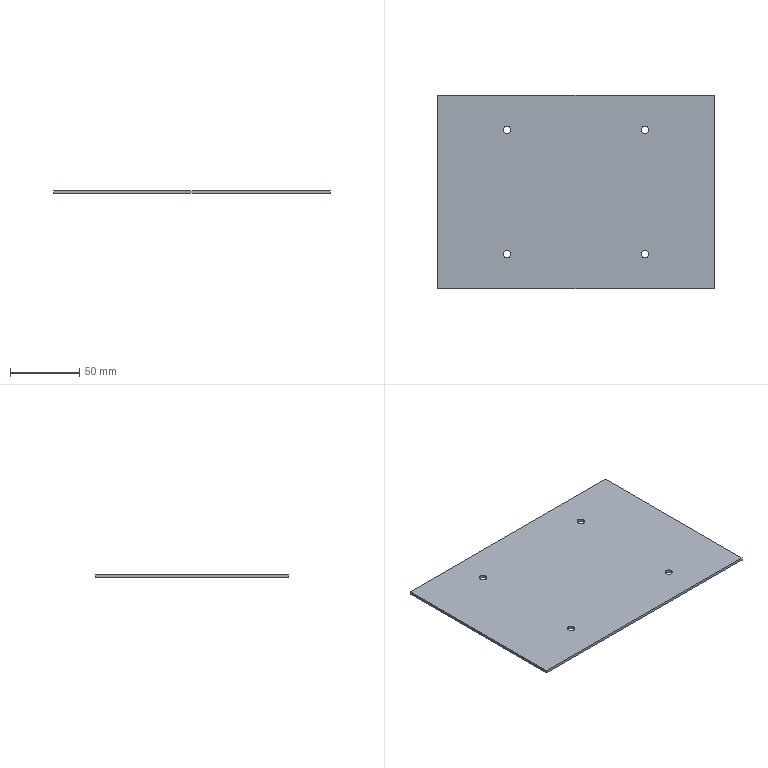Part | STEP file | SX-S36 | 1 solid | 14 faces | box 200 x 140 x 2 mm | volume 55817 mm3 | cylinder 8 | plane 6 | commonest cylinder face diameters 5.4 x8
STEP:
#1=CARTESIAN_POINT('',(0.,0.,0.));
#2=DIRECTION('',(0.,0.,1.));
#3=DIRECTION('',(1.,0.,0.));
#4=AXIS2_PLACEMENT_3D('',#1,#2,#3);
#5=CARTESIAN_POINT('',(-1471.912,1227.706,-2.));
#6=VERTEX_POINT('',#5);
#7=CARTESIAN_POINT('',(-1471.912,1227.706,0.));
#8=VERTEX_POINT('',#7);
#9=CARTESIAN_POINT('',(-1471.912,1227.706,-2.));
#10=DIRECTION('',(0.,0.,1.));
#11=VECTOR('',#10,1.);
#12=LINE('',#9,#11);
#13=CARTESIAN_POINT('',(-1474.612,1227.706,-2.));
#14=DIRECTION('',(0.,0.,1.));
#15=DIRECTION('',(1.,0.,0.));
#16=AXIS2_PLACEMENT_3D('',#13,#14,#15);
#17=CYLINDRICAL_SURFACE('',#16,2.7);
#18=CARTESIAN_POINT('',(6.283,0.));
#19=DIRECTION('',(0.,1.));
#20=VECTOR('',#19,1.);
#21=LINE('',#18,#20);
#22=(GEOMETRIC_REPRESENTATION_CONTEXT(2)PARAMETRIC_REPRESENTATION_CONTEXT()REPRESENTATION_CONTEXT('',''));
#23=DEFINITIONAL_REPRESENTATION('',(#21),#22);
#24=PCURVE('',#17,#23);
#25=CARTESIAN_POINT('',(-1474.612,1227.706,-2.));
#26=DIRECTION('',(0.,0.,1.));
#27=DIRECTION('',(1.,0.,0.));
#28=AXIS2_PLACEMENT_3D('',#25,#26,#27);
#29=CYLINDRICAL_SURFACE('',#28,2.7);
#30=CARTESIAN_POINT('',(0.,0.));
#31=DIRECTION('',(0.,1.));
#32=VECTOR('',#31,1.);
#33=LINE('',#30,#32);
#34=(GEOMETRIC_REPRESENTATION_CONTEXT(2)PARAMETRIC_REPRESENTATION_CONTEXT()REPRESENTATION_CONTEXT('',''));
#35=DEFINITIONAL_REPRESENTATION('',(#33),#34);
#36=PCURVE('',#29,#35);
#37=SURFACE_CURVE('',#12,(#24,#36),.PCURVE_S1.);
#38=EDGE_CURVE('',#6,#8,#37,.T.);
#39=ORIENTED_EDGE('',*,*,#38,.T.);
#40=CARTESIAN_POINT('',(-1477.312,1227.706,0.));
#41=VERTEX_POINT('',#40);
#42=CARTESIAN_POINT('',(-1474.612,1227.706,0.));
#43=DIRECTION('',(0.,0.,1.));
#44=DIRECTION('',(-1.,0.,0.));
#45=AXIS2_PLACEMENT_3D('',#42,#43,#44);
#46=CIRCLE('',#45,2.7);
#47=CARTESIAN_POINT('',(3.142,2.));
#48=DIRECTION('',(1.,0.));
#49=VECTOR('',#48,1.);
#50=LINE('',#47,#49);
#51=(GEOMETRIC_REPRESENTATION_CONTEXT(2)PARAMETRIC_REPRESENTATION_CONTEXT()REPRESENTATION_CONTEXT('',''));
#52=DEFINITIONAL_REPRESENTATION('',(#50),#51);
#53=PCURVE('',#17,#52);
#54=CARTESIAN_POINT('',(0.,0.,0.));
#55=DIRECTION('',(0.,0.,1.));
#56=DIRECTION('',(1.,0.,0.));
#57=AXIS2_PLACEMENT_3D('',#54,#55,#56);
#58=PLANE('',#57);
#59=CARTESIAN_POINT('',(-1474.612,1227.706));
#60=DIRECTION('',(-1.,0.));
#61=AXIS2_PLACEMENT_2D('',#59,#60);
#62=CIRCLE('',#61,2.7);
#63=(GEOMETRIC_REPRESENTATION_CONTEXT(2)PARAMETRIC_REPRESENTATION_CONTEXT()REPRESENTATION_CONTEXT('',''));
#64=DEFINITIONAL_REPRESENTATION('',(#62),#63);
#65=PCURVE('',#58,#64);
#66=SURFACE_CURVE('',#46,(#53,#65),.PCURVE_S1.);
#67=EDGE_CURVE('',#41,#8,#66,.T.);
#68=ORIENTED_EDGE('',*,*,#67,.F.);
#69=CARTESIAN_POINT('',(-1477.312,1227.706,-2.));
#70=VERTEX_POINT('',#69);
#71=CARTESIAN_POINT('',(-1477.312,1227.706,-2.));
#72=DIRECTION('',(0.,0.,1.));
#73=VECTOR('',#72,1.);
#74=LINE('',#71,#73);
#75=CARTESIAN_POINT('',(3.142,0.));
#76=DIRECTION('',(0.,1.));
#77=VECTOR('',#76,1.);
#78=LINE('',#75,#77);
#79=(GEOMETRIC_REPRESENTATION_CONTEXT(2)PARAMETRIC_REPRESENTATION_CONTEXT()REPRESENTATION_CONTEXT('',''));
#80=DEFINITIONAL_REPRESENTATION('',(#78),#79);
#81=PCURVE('',#17,#80);
#82=CARTESIAN_POINT('',(3.142,0.));
#83=DIRECTION('',(0.,1.));
#84=VECTOR('',#83,1.);
#85=LINE('',#82,#84);
#86=(GEOMETRIC_REPRESENTATION_CONTEXT(2)PARAMETRIC_REPRESENTATION_CONTEXT()REPRESENTATION_CONTEXT('',''));
#87=DEFINITIONAL_REPRESENTATION('',(#85),#86);
#88=PCURVE('',#29,#87);
#89=SURFACE_CURVE('',#74,(#81,#88),.PCURVE_S1.);
#90=EDGE_CURVE('',#70,#41,#89,.T.);
#91=ORIENTED_EDGE('',*,*,#90,.F.);
#92=CARTESIAN_POINT('',(-1474.612,1227.706,-2.));
#93=DIRECTION('',(0.,0.,1.));
#94=DIRECTION('',(-1.,0.,0.));
#95=AXIS2_PLACEMENT_3D('',#92,#93,#94);
#96=CIRCLE('',#95,2.7);
#97=CARTESIAN_POINT('',(3.142,0.));
#98=DIRECTION('',(1.,0.));
#99=VECTOR('',#98,1.);
#100=LINE('',#97,#99);
#101=(GEOMETRIC_REPRESENTATION_CONTEXT(2)PARAMETRIC_REPRESENTATION_CONTEXT()REPRESENTATION_CONTEXT('',''));
#102=DEFINITIONAL_REPRESENTATION('',(#100),#101);
#103=PCURVE('',#17,#102);
#104=CARTESIAN_POINT('',(0.,0.,-2.));
#105=DIRECTION('',(0.,0.,1.));
#106=DIRECTION('',(1.,0.,0.));
#107=AXIS2_PLACEMENT_3D('',#104,#105,#106);
#108=PLANE('',#107);
#109=CARTESIAN_POINT('',(-1474.612,1227.706));
#110=DIRECTION('',(-1.,0.));
#111=AXIS2_PLACEMENT_2D('',#109,#110);
#112=CIRCLE('',#111,2.7);
#113=(GEOMETRIC_REPRESENTATION_CONTEXT(2)PARAMETRIC_REPRESENTATION_CONTEXT()REPRESENTATION_CONTEXT('',''));
#114=DEFINITIONAL_REPRESENTATION('',(#112),#113);
#115=PCURVE('',#108,#114);
#116=SURFACE_CURVE('',#96,(#103,#115),.PCURVE_S1.);
#117=EDGE_CURVE('',#70,#6,#116,.T.);
#118=ORIENTED_EDGE('',*,*,#117,.T.);
#119=EDGE_LOOP('',(#39,#68,#91,#118));
#120=FACE_BOUND('',#119,.F.);
#121=ADVANCED_FACE('',(#120),#17,.F.);
#122=CARTESIAN_POINT('',(-1471.912,1137.706,-2.));
#123=VERTEX_POINT('',#122);
#124=CARTESIAN_POINT('',(-1471.912,1137.706,0.));
#125=VERTEX_POINT('',#124);
#126=CARTESIAN_POINT('',(-1471.912,1137.706,-2.));
#127=DIRECTION('',(0.,0.,1.));
#128=VECTOR('',#127,1.);
#129=LINE('',#126,#128);
#130=CARTESIAN_POINT('',(-1474.612,1137.706,-2.));
#131=DIRECTION('',(0.,0.,1.));
#132=DIRECTION('',(1.,0.,0.));
#133=AXIS2_PLACEMENT_3D('',#130,#131,#132);
#134=CYLINDRICAL_SURFACE('',#133,2.7);
#135=CARTESIAN_POINT('',(6.283,0.));
#136=DIRECTION('',(0.,1.));
#137=VECTOR('',#136,1.);
#138=LINE('',#135,#137);
#139=(GEOMETRIC_REPRESENTATION_CONTEXT(2)PARAMETRIC_REPRESENTATION_CONTEXT()REPRESENTATION_CONTEXT('',''));
#140=DEFINITIONAL_REPRESENTATION('',(#138),#139);
#141=PCURVE('',#134,#140);
#142=CARTESIAN_POINT('',(-1474.612,1137.706,-2.));
#143=DIRECTION('',(0.,0.,1.));
#144=DIRECTION('',(1.,0.,0.));
#145=AXIS2_PLACEMENT_3D('',#142,#143,#144);
#146=CYLINDRICAL_SURFACE('',#145,2.7);
#147=CARTESIAN_POINT('',(0.,0.));
#148=DIRECTION('',(0.,1.));
#149=VECTOR('',#148,1.);
#150=LINE('',#147,#149);
#151=(GEOMETRIC_REPRESENTATION_CONTEXT(2)PARAMETRIC_REPRESENTATION_CONTEXT()REPRESENTATION_CONTEXT('',''));
#152=DEFINITIONAL_REPRESENTATION('',(#150),#151);
#153=PCURVE('',#146,#152);
#154=SURFACE_CURVE('',#129,(#141,#153),.PCURVE_S1.);
#155=EDGE_CURVE('',#123,#125,#154,.T.);
#156=ORIENTED_EDGE('',*,*,#155,.T.);
#157=CARTESIAN_POINT('',(-1477.312,1137.706,0.));
#158=VERTEX_POINT('',#157);
#159=CARTESIAN_POINT('',(-1474.612,1137.706,0.));
#160=DIRECTION('',(0.,0.,1.));
#161=DIRECTION('',(1.,0.,0.));
#162=AXIS2_PLACEMENT_3D('',#159,#160,#161);
#163=CIRCLE('',#162,2.7);
#164=CARTESIAN_POINT('',(0.,2.));
#165=DIRECTION('',(1.,0.));
#166=VECTOR('',#165,1.);
#167=LINE('',#164,#166);
#168=(GEOMETRIC_REPRESENTATION_CONTEXT(2)PARAMETRIC_REPRESENTATION_CONTEXT()REPRESENTATION_CONTEXT('',''));
#169=DEFINITIONAL_REPRESENTATION('',(#167),#168);
#170=PCURVE('',#134,#169);
#171=CARTESIAN_POINT('',(-1474.612,1137.706));
#172=DIRECTION('',(1.,0.));
#173=AXIS2_PLACEMENT_2D('',#171,#172);
#174=CIRCLE('',#173,2.7);
#175=(GEOMETRIC_REPRESENTATION_CONTEXT(2)PARAMETRIC_REPRESENTATION_CONTEXT()REPRESENTATION_CONTEXT('',''));
#176=DEFINITIONAL_REPRESENTATION('',(#174),#175);
#177=PCURVE('',#58,#176);
#178=SURFACE_CURVE('',#163,(#170,#177),.PCURVE_S1.);
#179=EDGE_CURVE('',#158,#125,#178,.T.);
#180=ORIENTED_EDGE('',*,*,#179,.F.);
#181=CARTESIAN_POINT('',(-1477.312,1137.706,-2.));
#182=VERTEX_POINT('',#181);
#183=CARTESIAN_POINT('',(-1477.312,1137.706,-2.));
#184=DIRECTION('',(0.,0.,1.));
#185=VECTOR('',#184,1.);
#186=LINE('',#183,#185);
#187=CARTESIAN_POINT('',(3.142,0.));
#188=DIRECTION('',(0.,1.));
#189=VECTOR('',#188,1.);
#190=LINE('',#187,#189);
#191=(GEOMETRIC_REPRESENTATION_CONTEXT(2)PARAMETRIC_REPRESENTATION_CONTEXT()REPRESENTATION_CONTEXT('',''));
#192=DEFINITIONAL_REPRESENTATION('',(#190),#191);
#193=PCURVE('',#134,#192);
#194=CARTESIAN_POINT('',(3.142,0.));
#195=DIRECTION('',(0.,1.));
#196=VECTOR('',#195,1.);
#197=LINE('',#194,#196);
#198=(GEOMETRIC_REPRESENTATION_CONTEXT(2)PARAMETRIC_REPRESENTATION_CONTEXT()REPRESENTATION_CONTEXT('',''));
#199=DEFINITIONAL_REPRESENTATION('',(#197),#198);
#200=PCURVE('',#146,#199);
#201=SURFACE_CURVE('',#186,(#193,#200),.PCURVE_S1.);
#202=EDGE_CURVE('',#182,#158,#201,.T.);
#203=ORIENTED_EDGE('',*,*,#202,.F.);
#204=CARTESIAN_POINT('',(-1474.612,1137.706,-2.));
#205=DIRECTION('',(0.,0.,1.));
#206=DIRECTION('',(1.,0.,0.));
#207=AXIS2_PLACEMENT_3D('',#204,#205,#206);
#208=CIRCLE('',#207,2.7);
#209=CARTESIAN_POINT('',(0.,0.));
#210=DIRECTION('',(1.,0.));
#211=VECTOR('',#210,1.);
#212=LINE('',#209,#211);
#213=(GEOMETRIC_REPRESENTATION_CONTEXT(2)PARAMETRIC_REPRESENTATION_CONTEXT()REPRESENTATION_CONTEXT('',''));
#214=DEFINITIONAL_REPRESENTATION('',(#212),#213);
#215=PCURVE('',#134,#214);
#216=CARTESIAN_POINT('',(-1474.612,1137.706));
#217=DIRECTION('',(1.,0.));
#218=AXIS2_PLACEMENT_2D('',#216,#217);
#219=CIRCLE('',#218,2.7);
#220=(GEOMETRIC_REPRESENTATION_CONTEXT(2)PARAMETRIC_REPRESENTATION_CONTEXT()REPRESENTATION_CONTEXT('',''));
#221=DEFINITIONAL_REPRESENTATION('',(#219),#220);
#222=PCURVE('',#108,#221);
#223=SURFACE_CURVE('',#208,(#215,#222),.PCURVE_S1.);
#224=EDGE_CURVE('',#182,#123,#223,.T.);
#225=ORIENTED_EDGE('',*,*,#224,.T.);
#226=EDGE_LOOP('',(#156,#180,#203,#225));
#227=FACE_BOUND('',#226,.F.);
#228=ADVANCED_FACE('',(#227),#134,.F.);
#229=CARTESIAN_POINT('',(-1571.912,1137.706,-2.));
#230=VERTEX_POINT('',#229);
#231=CARTESIAN_POINT('',(-1571.912,1137.706,0.));
#232=VERTEX_POINT('',#231);
#233=CARTESIAN_POINT('',(-1571.912,1137.706,-2.));
#234=DIRECTION('',(0.,0.,1.));
#235=VECTOR('',#234,1.);
#236=LINE('',#233,#235);
#237=CARTESIAN_POINT('',(-1574.612,1137.706,-2.));
#238=DIRECTION('',(0.,0.,1.));
#239=DIRECTION('',(1.,0.,0.));
#240=AXIS2_PLACEMENT_3D('',#237,#238,#239);
#241=CYLINDRICAL_SURFACE('',#240,2.7);
#242=CARTESIAN_POINT('',(6.283,0.));
#243=DIRECTION('',(0.,1.));
#244=VECTOR('',#243,1.);
#245=LINE('',#242,#244);
#246=(GEOMETRIC_REPRESENTATION_CONTEXT(2)PARAMETRIC_REPRESENTATION_CONTEXT()REPRESENTATION_CONTEXT('',''));
#247=DEFINITIONAL_REPRESENTATION('',(#245),#246);
#248=PCURVE('',#241,#247);
#249=CARTESIAN_POINT('',(-1574.612,1137.706,-2.));
#250=DIRECTION('',(0.,0.,1.));
#251=DIRECTION('',(1.,0.,0.));
#252=AXIS2_PLACEMENT_3D('',#249,#250,#251);
#253=CYLINDRICAL_SURFACE('',#252,2.7);
#254=CARTESIAN_POINT('',(0.,0.));
#255=DIRECTION('',(0.,1.));
#256=VECTOR('',#255,1.);
#257=LINE('',#254,#256);
#258=(GEOMETRIC_REPRESENTATION_CONTEXT(2)PARAMETRIC_REPRESENTATION_CONTEXT()REPRESENTATION_CONTEXT('',''));
#259=DEFINITIONAL_REPRESENTATION('',(#257),#258);
#260=PCURVE('',#253,#259);
#261=SURFACE_CURVE('',#236,(#248,#260),.PCURVE_S1.);
#262=EDGE_CURVE('',#230,#232,#261,.T.);
#263=ORIENTED_EDGE('',*,*,#262,.T.);
#264=CARTESIAN_POINT('',(-1577.312,1137.706,0.));
#265=VERTEX_POINT('',#264);
#266=CARTESIAN_POINT('',(-1574.612,1137.706,0.));
#267=DIRECTION('',(0.,0.,1.));
#268=DIRECTION('',(-1.,0.,0.));
#269=AXIS2_PLACEMENT_3D('',#266,#267,#268);
#270=CIRCLE('',#269,2.7);
#271=CARTESIAN_POINT('',(3.142,2.));
#272=DIRECTION('',(1.,0.));
#273=VECTOR('',#272,1.);
#274=LINE('',#271,#273);
#275=(GEOMETRIC_REPRESENTATION_CONTEXT(2)PARAMETRIC_REPRESENTATION_CONTEXT()REPRESENTATION_CONTEXT('',''));
#276=DEFINITIONAL_REPRESENTATION('',(#274),#275);
#277=PCURVE('',#241,#276);
#278=CARTESIAN_POINT('',(-1574.612,1137.706));
#279=DIRECTION('',(-1.,0.));
#280=AXIS2_PLACEMENT_2D('',#278,#279);
#281=CIRCLE('',#280,2.7);
#282=(GEOMETRIC_REPRESENTATION_CONTEXT(2)PARAMETRIC_REPRESENTATION_CONTEXT()REPRESENTATION_CONTEXT('',''));
#283=DEFINITIONAL_REPRESENTATION('',(#281),#282);
#284=PCURVE('',#58,#283);
#285=SURFACE_CURVE('',#270,(#277,#284),.PCURVE_S1.);
#286=EDGE_CURVE('',#265,#232,#285,.T.);
#287=ORIENTED_EDGE('',*,*,#286,.F.);
#288=CARTESIAN_POINT('',(-1577.312,1137.706,-2.));
#289=VERTEX_POINT('',#288);
#290=CARTESIAN_POINT('',(-1577.312,1137.706,-2.));
#291=DIRECTION('',(0.,0.,1.));
#292=VECTOR('',#291,1.);
#293=LINE('',#290,#292);
#294=CARTESIAN_POINT('',(3.142,0.));
#295=DIRECTION('',(0.,1.));
#296=VECTOR('',#295,1.);
#297=LINE('',#294,#296);
#298=(GEOMETRIC_REPRESENTATION_CONTEXT(2)PARAMETRIC_REPRESENTATION_CONTEXT()REPRESENTATION_CONTEXT('',''));
#299=DEFINITIONAL_REPRESENTATION('',(#297),#298);
#300=PCURVE('',#241,#299);
#301=CARTESIAN_POINT('',(3.142,0.));
#302=DIRECTION('',(0.,1.));
#303=VECTOR('',#302,1.);
#304=LINE('',#301,#303);
#305=(GEOMETRIC_REPRESENTATION_CONTEXT(2)PARAMETRIC_REPRESENTATION_CONTEXT()REPRESENTATION_CONTEXT('',''));
#306=DEFINITIONAL_REPRESENTATION('',(#304),#305);
#307=PCURVE('',#253,#306);
#308=SURFACE_CURVE('',#293,(#300,#307),.PCURVE_S1.);
#309=EDGE_CURVE('',#289,#265,#308,.T.);
#310=ORIENTED_EDGE('',*,*,#309,.F.);
#311=CARTESIAN_POINT('',(-1574.612,1137.706,-2.));
#312=DIRECTION('',(0.,0.,1.));
#313=DIRECTION('',(-1.,0.,0.));
#314=AXIS2_PLACEMENT_3D('',#311,#312,#313);
#315=CIRCLE('',#314,2.7);
#316=CARTESIAN_POINT('',(3.142,0.));
#317=DIRECTION('',(1.,0.));
#318=VECTOR('',#317,1.);
#319=LINE('',#316,#318);
#320=(GEOMETRIC_REPRESENTATION_CONTEXT(2)PARAMETRIC_REPRESENTATION_CONTEXT()REPRESENTATION_CONTEXT('',''));
#321=DEFINITIONAL_REPRESENTATION('',(#319),#320);
#322=PCURVE('',#241,#321);
#323=CARTESIAN_POINT('',(-1574.612,1137.706));
#324=DIRECTION('',(-1.,0.));
#325=AXIS2_PLACEMENT_2D('',#323,#324);
#326=CIRCLE('',#325,2.7);
#327=(GEOMETRIC_REPRESENTATION_CONTEXT(2)PARAMETRIC_REPRESENTATION_CONTEXT()REPRESENTATION_CONTEXT('',''));
#328=DEFINITIONAL_REPRESENTATION('',(#326),#327);
#329=PCURVE('',#108,#328);
#330=SURFACE_CURVE('',#315,(#322,#329),.PCURVE_S1.);
#331=EDGE_CURVE('',#289,#230,#330,.T.);
#332=ORIENTED_EDGE('',*,*,#331,.T.);
#333=EDGE_LOOP('',(#263,#287,#310,#332));
#334=FACE_BOUND('',#333,.F.);
#335=ADVANCED_FACE('',(#334),#241,.F.);
#336=CARTESIAN_POINT('',(-1571.912,1227.706,-2.));
#337=VERTEX_POINT('',#336);
#338=CARTESIAN_POINT('',(-1571.912,1227.706,0.));
#339=VERTEX_POINT('',#338);
#340=CARTESIAN_POINT('',(-1571.912,1227.706,-2.));
#341=DIRECTION('',(0.,0.,1.));
#342=VECTOR('',#341,1.);
#343=LINE('',#340,#342);
#344=CARTESIAN_POINT('',(-1574.612,1227.706,-2.));
#345=DIRECTION('',(0.,0.,1.));
#346=DIRECTION('',(1.,0.,0.));
#347=AXIS2_PLACEMENT_3D('',#344,#345,#346);
#348=CYLINDRICAL_SURFACE('',#347,2.7);
#349=CARTESIAN_POINT('',(6.283,0.));
#350=DIRECTION('',(0.,1.));
#351=VECTOR('',#350,1.);
#352=LINE('',#349,#351);
#353=(GEOMETRIC_REPRESENTATION_CONTEXT(2)PARAMETRIC_REPRESENTATION_CONTEXT()REPRESENTATION_CONTEXT('',''));
#354=DEFINITIONAL_REPRESENTATION('',(#352),#353);
#355=PCURVE('',#348,#354);
#356=CARTESIAN_POINT('',(-1574.612,1227.706,-2.));
#357=DIRECTION('',(0.,0.,1.));
#358=DIRECTION('',(1.,0.,0.));
#359=AXIS2_PLACEMENT_3D('',#356,#357,#358);
#360=CYLINDRICAL_SURFACE('',#359,2.7);
#361=CARTESIAN_POINT('',(0.,0.));
#362=DIRECTION('',(0.,1.));
#363=VECTOR('',#362,1.);
#364=LINE('',#361,#363);
#365=(GEOMETRIC_REPRESENTATION_CONTEXT(2)PARAMETRIC_REPRESENTATION_CONTEXT()REPRESENTATION_CONTEXT('',''));
#366=DEFINITIONAL_REPRESENTATION('',(#364),#365);
#367=PCURVE('',#360,#366);
#368=SURFACE_CURVE('',#343,(#355,#367),.PCURVE_S1.);
#369=EDGE_CURVE('',#337,#339,#368,.T.);
#370=ORIENTED_EDGE('',*,*,#369,.T.);
#371=CARTESIAN_POINT('',(-1577.312,1227.706,0.));
#372=VERTEX_POINT('',#371);
#373=CARTESIAN_POINT('',(-1574.612,1227.706,0.));
#374=DIRECTION('',(0.,0.,1.));
#375=DIRECTION('',(1.,0.,0.));
#376=AXIS2_PLACEMENT_3D('',#373,#374,#375);
#377=CIRCLE('',#376,2.7);
#378=CARTESIAN_POINT('',(0.,2.));
#379=DIRECTION('',(1.,0.));
#380=VECTOR('',#379,1.);
#381=LINE('',#378,#380);
#382=(GEOMETRIC_REPRESENTATION_CONTEXT(2)PARAMETRIC_REPRESENTATION_CONTEXT()REPRESENTATION_CONTEXT('',''));
#383=DEFINITIONAL_REPRESENTATION('',(#381),#382);
#384=PCURVE('',#348,#383);
#385=CARTESIAN_POINT('',(-1574.612,1227.706));
#386=DIRECTION('',(1.,0.));
#387=AXIS2_PLACEMENT_2D('',#385,#386);
#388=CIRCLE('',#387,2.7);
#389=(GEOMETRIC_REPRESENTATION_CONTEXT(2)PARAMETRIC_REPRESENTATION_CONTEXT()REPRESENTATION_CONTEXT('',''));
#390=DEFINITIONAL_REPRESENTATION('',(#388),#389);
#391=PCURVE('',#58,#390);
#392=SURFACE_CURVE('',#377,(#384,#391),.PCURVE_S1.);
#393=EDGE_CURVE('',#372,#339,#392,.T.);
#394=ORIENTED_EDGE('',*,*,#393,.F.);
#395=CARTESIAN_POINT('',(-1577.312,1227.706,-2.));
#396=VERTEX_POINT('',#395);
#397=CARTESIAN_POINT('',(-1577.312,1227.706,-2.));
#398=DIRECTION('',(0.,0.,1.));
#399=VECTOR('',#398,1.);
#400=LINE('',#397,#399);
#401=CARTESIAN_POINT('',(3.142,0.));
#402=DIRECTION('',(0.,1.));
#403=VECTOR('',#402,1.);
#404=LINE('',#401,#403);
#405=(GEOMETRIC_REPRESENTATION_CONTEXT(2)PARAMETRIC_REPRESENTATION_CONTEXT()REPRESENTATION_CONTEXT('',''));
#406=DEFINITIONAL_REPRESENTATION('',(#404),#405);
#407=PCURVE('',#348,#406);
#408=CARTESIAN_POINT('',(3.142,0.));
#409=DIRECTION('',(0.,1.));
#410=VECTOR('',#409,1.);
#411=LINE('',#408,#410);
#412=(GEOMETRIC_REPRESENTATION_CONTEXT(2)PARAMETRIC_REPRESENTATION_CONTEXT()REPRESENTATION_CONTEXT('',''));
#413=DEFINITIONAL_REPRESENTATION('',(#411),#412);
#414=PCURVE('',#360,#413);
#415=SURFACE_CURVE('',#400,(#407,#414),.PCURVE_S1.);
#416=EDGE_CURVE('',#396,#372,#415,.T.);
#417=ORIENTED_EDGE('',*,*,#416,.F.);
#418=CARTESIAN_POINT('',(-1574.612,1227.706,-2.));
#419=DIRECTION('',(0.,0.,1.));
#420=DIRECTION('',(1.,0.,0.));
#421=AXIS2_PLACEMENT_3D('',#418,#419,#420);
#422=CIRCLE('',#421,2.7);
#423=CARTESIAN_POINT('',(0.,0.));
#424=DIRECTION('',(1.,0.));
#425=VECTOR('',#424,1.);
#426=LINE('',#423,#425);
#427=(GEOMETRIC_REPRESENTATION_CONTEXT(2)PARAMETRIC_REPRESENTATION_CONTEXT()REPRESENTATION_CONTEXT('',''));
#428=DEFINITIONAL_REPRESENTATION('',(#426),#427);
#429=PCURVE('',#348,#428);
#430=CARTESIAN_POINT('',(-1574.612,1227.706));
#431=DIRECTION('',(1.,0.));
#432=AXIS2_PLACEMENT_2D('',#430,#431);
#433=CIRCLE('',#432,2.7);
#434=(GEOMETRIC_REPRESENTATION_CONTEXT(2)PARAMETRIC_REPRESENTATION_CONTEXT()REPRESENTATION_CONTEXT('',''));
#435=DEFINITIONAL_REPRESENTATION('',(#433),#434);
#436=PCURVE('',#108,#435);
#437=SURFACE_CURVE('',#422,(#429,#436),.PCURVE_S1.);
#438=EDGE_CURVE('',#396,#337,#437,.T.);
#439=ORIENTED_EDGE('',*,*,#438,.T.);
#440=EDGE_LOOP('',(#370,#394,#417,#439));
#441=FACE_BOUND('',#440,.F.);
#442=ADVANCED_FACE('',(#441),#348,.F.);
#443=CARTESIAN_POINT('',(-1624.612,1252.706,0.));
#444=VERTEX_POINT('',#443);
#445=CARTESIAN_POINT('',(-1624.612,1112.706,0.));
#446=VERTEX_POINT('',#445);
#447=CARTESIAN_POINT('',(-1624.612,1252.706,0.));
#448=DIRECTION('',(0.,-1.,0.));
#449=VECTOR('',#448,1.);
#450=LINE('',#447,#449);
#451=CARTESIAN_POINT('',(-1624.612,1252.706,-2.));
#452=DIRECTION('',(-1.,0.,0.));
#453=DIRECTION('',(0.,0.,1.));
#454=AXIS2_PLACEMENT_3D('',#451,#452,#453);
#455=PLANE('',#454);
#456=CARTESIAN_POINT('',(2.,0.));
#457=DIRECTION('',(0.,-1.));
#458=VECTOR('',#457,1.);
#459=LINE('',#456,#458);
#460=(GEOMETRIC_REPRESENTATION_CONTEXT(2)PARAMETRIC_REPRESENTATION_CONTEXT()REPRESENTATION_CONTEXT('',''));
#461=DEFINITIONAL_REPRESENTATION('',(#459),#460);
#462=PCURVE('',#455,#461);
#463=CARTESIAN_POINT('',(-1624.612,1252.706));
#464=DIRECTION('',(0.,-1.));
#465=VECTOR('',#464,1.);
#466=LINE('',#463,#465);
#467=(GEOMETRIC_REPRESENTATION_CONTEXT(2)PARAMETRIC_REPRESENTATION_CONTEXT()REPRESENTATION_CONTEXT('',''));
#468=DEFINITIONAL_REPRESENTATION('',(#466),#467);
#469=PCURVE('',#58,#468);
#470=SURFACE_CURVE('',#450,(#462,#469),.PCURVE_S1.);
#471=EDGE_CURVE('',#444,#446,#470,.T.);
#472=ORIENTED_EDGE('',*,*,#471,.F.);
#473=CARTESIAN_POINT('',(-1624.612,1252.706,-2.));
#474=VERTEX_POINT('',#473);
#475=CARTESIAN_POINT('',(-1624.612,1252.706,-2.));
#476=DIRECTION('',(0.,0.,1.));
#477=VECTOR('',#476,1.);
#478=LINE('',#475,#477);
#479=CARTESIAN_POINT('',(0.,0.));
#480=DIRECTION('',(1.,0.));
#481=VECTOR('',#480,1.);
#482=LINE('',#479,#481);
#483=(GEOMETRIC_REPRESENTATION_CONTEXT(2)PARAMETRIC_REPRESENTATION_CONTEXT()REPRESENTATION_CONTEXT('',''));
#484=DEFINITIONAL_REPRESENTATION('',(#482),#483);
#485=PCURVE('',#455,#484);
#486=CARTESIAN_POINT('',(-1624.612,1252.706,-2.));
#487=DIRECTION('',(0.,1.,0.));
#488=DIRECTION('',(0.,0.,1.));
#489=AXIS2_PLACEMENT_3D('',#486,#487,#488);
#490=PLANE('',#489);
#491=CARTESIAN_POINT('',(0.,0.));
#492=DIRECTION('',(1.,0.));
#493=VECTOR('',#492,1.);
#494=LINE('',#491,#493);
#495=(GEOMETRIC_REPRESENTATION_CONTEXT(2)PARAMETRIC_REPRESENTATION_CONTEXT()REPRESENTATION_CONTEXT('',''));
#496=DEFINITIONAL_REPRESENTATION('',(#494),#495);
#497=PCURVE('',#490,#496);
#498=SURFACE_CURVE('',#478,(#485,#497),.PCURVE_S1.);
#499=EDGE_CURVE('',#474,#444,#498,.T.);
#500=ORIENTED_EDGE('',*,*,#499,.F.);
#501=CARTESIAN_POINT('',(-1624.612,1112.706,-2.));
#502=VERTEX_POINT('',#501);
#503=CARTESIAN_POINT('',(-1624.612,1252.706,-2.));
#504=DIRECTION('',(0.,-1.,0.));
#505=VECTOR('',#504,1.);
#506=LINE('',#503,#505);
#507=CARTESIAN_POINT('',(0.,0.));
#508=DIRECTION('',(0.,-1.));
#509=VECTOR('',#508,1.);
#510=LINE('',#507,#509);
#511=(GEOMETRIC_REPRESENTATION_CONTEXT(2)PARAMETRIC_REPRESENTATION_CONTEXT()REPRESENTATION_CONTEXT('',''));
#512=DEFINITIONAL_REPRESENTATION('',(#510),#511);
#513=PCURVE('',#455,#512);
#514=CARTESIAN_POINT('',(-1624.612,1252.706));
#515=DIRECTION('',(0.,-1.));
#516=VECTOR('',#515,1.);
#517=LINE('',#514,#516);
#518=(GEOMETRIC_REPRESENTATION_CONTEXT(2)PARAMETRIC_REPRESENTATION_CONTEXT()REPRESENTATION_CONTEXT('',''));
#519=DEFINITIONAL_REPRESENTATION('',(#517),#518);
#520=PCURVE('',#108,#519);
#521=SURFACE_CURVE('',#506,(#513,#520),.PCURVE_S1.);
#522=EDGE_CURVE('',#474,#502,#521,.T.);
#523=ORIENTED_EDGE('',*,*,#522,.T.);
#524=CARTESIAN_POINT('',(-1624.612,1112.706,-2.));
#525=DIRECTION('',(0.,0.,1.));
#526=VECTOR('',#525,1.);
#527=LINE('',#524,#526);
#528=CARTESIAN_POINT('',(0.,-140.));
#529=DIRECTION('',(1.,0.));
#530=VECTOR('',#529,1.);
#531=LINE('',#528,#530);
#532=(GEOMETRIC_REPRESENTATION_CONTEXT(2)PARAMETRIC_REPRESENTATION_CONTEXT()REPRESENTATION_CONTEXT('',''));
#533=DEFINITIONAL_REPRESENTATION('',(#531),#532);
#534=PCURVE('',#455,#533);
#535=CARTESIAN_POINT('',(-1624.612,1112.706,-2.));
#536=DIRECTION('',(0.,-1.,0.));
#537=DIRECTION('',(0.,0.,-1.));
#538=AXIS2_PLACEMENT_3D('',#535,#536,#537);
#539=PLANE('',#538);
#540=CARTESIAN_POINT('',(0.,0.));
#541=DIRECTION('',(-1.,0.));
#542=VECTOR('',#541,1.);
#543=LINE('',#540,#542);
#544=(GEOMETRIC_REPRESENTATION_CONTEXT(2)PARAMETRIC_REPRESENTATION_CONTEXT()REPRESENTATION_CONTEXT('',''));
#545=DEFINITIONAL_REPRESENTATION('',(#543),#544);
#546=PCURVE('',#539,#545);
#547=SURFACE_CURVE('',#527,(#534,#546),.PCURVE_S1.);
#548=EDGE_CURVE('',#502,#446,#547,.T.);
#549=ORIENTED_EDGE('',*,*,#548,.T.);
#550=EDGE_LOOP('',(#472,#500,#523,#549));
#551=FACE_BOUND('',#550,.T.);
#552=ADVANCED_FACE('',(#551),#455,.T.);
#553=CARTESIAN_POINT('',(-1424.612,1252.706,0.));
#554=VERTEX_POINT('',#553);
#555=CARTESIAN_POINT('',(-1624.612,1252.706,0.));
#556=DIRECTION('',(-1.,0.,0.));
#557=VECTOR('',#556,1.);
#558=LINE('',#555,#557);
#559=CARTESIAN_POINT('',(2.,0.));
#560=DIRECTION('',(0.,-1.));
#561=VECTOR('',#560,1.);
#562=LINE('',#559,#561);
#563=(GEOMETRIC_REPRESENTATION_CONTEXT(2)PARAMETRIC_REPRESENTATION_CONTEXT()REPRESENTATION_CONTEXT('',''));
#564=DEFINITIONAL_REPRESENTATION('',(#562),#563);
#565=PCURVE('',#490,#564);
#566=CARTESIAN_POINT('',(-1624.612,1252.706));
#567=DIRECTION('',(-1.,0.));
#568=VECTOR('',#567,1.);
#569=LINE('',#566,#568);
#570=(GEOMETRIC_REPRESENTATION_CONTEXT(2)PARAMETRIC_REPRESENTATION_CONTEXT()REPRESENTATION_CONTEXT('',''));
#571=DEFINITIONAL_REPRESENTATION('',(#569),#570);
#572=PCURVE('',#58,#571);
#573=SURFACE_CURVE('',#558,(#565,#572),.PCURVE_S1.);
#574=EDGE_CURVE('',#554,#444,#573,.T.);
#575=ORIENTED_EDGE('',*,*,#574,.F.);
#576=CARTESIAN_POINT('',(-1424.612,1252.706,-2.));
#577=VERTEX_POINT('',#576);
#578=CARTESIAN_POINT('',(-1424.612,1252.706,-2.));
#579=DIRECTION('',(0.,0.,1.));
#580=VECTOR('',#579,1.);
#581=LINE('',#578,#580);
#582=CARTESIAN_POINT('',(0.,200.));
#583=DIRECTION('',(1.,0.));
#584=VECTOR('',#583,1.);
#585=LINE('',#582,#584);
#586=(GEOMETRIC_REPRESENTATION_CONTEXT(2)PARAMETRIC_REPRESENTATION_CONTEXT()REPRESENTATION_CONTEXT('',''));
#587=DEFINITIONAL_REPRESENTATION('',(#585),#586);
#588=PCURVE('',#490,#587);
#589=CARTESIAN_POINT('',(-1424.612,1252.706,-2.));
#590=DIRECTION('',(1.,0.,0.));
#591=DIRECTION('',(0.,0.,-1.));
#592=AXIS2_PLACEMENT_3D('',#589,#590,#591);
#593=PLANE('',#592);
#594=CARTESIAN_POINT('',(0.,0.));
#595=DIRECTION('',(-1.,0.));
#596=VECTOR('',#595,1.);
#597=LINE('',#594,#596);
#598=(GEOMETRIC_REPRESENTATION_CONTEXT(2)PARAMETRIC_REPRESENTATION_CONTEXT()REPRESENTATION_CONTEXT('',''));
#599=DEFINITIONAL_REPRESENTATION('',(#597),#598);
#600=PCURVE('',#593,#599);
#601=SURFACE_CURVE('',#581,(#588,#600),.PCURVE_S1.);
#602=EDGE_CURVE('',#577,#554,#601,.T.);
#603=ORIENTED_EDGE('',*,*,#602,.F.);
#604=CARTESIAN_POINT('',(-1624.612,1252.706,-2.));
#605=DIRECTION('',(-1.,0.,0.));
#606=VECTOR('',#605,1.);
#607=LINE('',#604,#606);
#608=CARTESIAN_POINT('',(0.,0.));
#609=DIRECTION('',(0.,-1.));
#610=VECTOR('',#609,1.);
#611=LINE('',#608,#610);
#612=(GEOMETRIC_REPRESENTATION_CONTEXT(2)PARAMETRIC_REPRESENTATION_CONTEXT()REPRESENTATION_CONTEXT('',''));
#613=DEFINITIONAL_REPRESENTATION('',(#611),#612);
#614=PCURVE('',#490,#613);
#615=CARTESIAN_POINT('',(-1624.612,1252.706));
#616=DIRECTION('',(-1.,0.));
#617=VECTOR('',#616,1.);
#618=LINE('',#615,#617);
#619=(GEOMETRIC_REPRESENTATION_CONTEXT(2)PARAMETRIC_REPRESENTATION_CONTEXT()REPRESENTATION_CONTEXT('',''));
#620=DEFINITIONAL_REPRESENTATION('',(#618),#619);
#621=PCURVE('',#108,#620);
#622=SURFACE_CURVE('',#607,(#614,#621),.PCURVE_S1.);
#623=EDGE_CURVE('',#577,#474,#622,.T.);
#624=ORIENTED_EDGE('',*,*,#623,.T.);
#625=ORIENTED_EDGE('',*,*,#499,.T.);
#626=EDGE_LOOP('',(#575,#603,#624,#625));
#627=FACE_BOUND('',#626,.T.);
#628=ADVANCED_FACE('',(#627),#490,.T.);
#629=CARTESIAN_POINT('',(-1424.612,1112.706,0.));
#630=VERTEX_POINT('',#629);
#631=CARTESIAN_POINT('',(-1424.612,1252.706,0.));
#632=DIRECTION('',(0.,1.,0.));
#633=VECTOR('',#632,1.);
#634=LINE('',#631,#633);
#635=CARTESIAN_POINT('',(-2.,0.));
#636=DIRECTION('',(0.,1.));
#637=VECTOR('',#636,1.);
#638=LINE('',#635,#637);
#639=(GEOMETRIC_REPRESENTATION_CONTEXT(2)PARAMETRIC_REPRESENTATION_CONTEXT()REPRESENTATION_CONTEXT('',''));
#640=DEFINITIONAL_REPRESENTATION('',(#638),#639);
#641=PCURVE('',#593,#640);
#642=CARTESIAN_POINT('',(-1424.612,1252.706));
#643=DIRECTION('',(0.,1.));
#644=VECTOR('',#643,1.);
#645=LINE('',#642,#644);
#646=(GEOMETRIC_REPRESENTATION_CONTEXT(2)PARAMETRIC_REPRESENTATION_CONTEXT()REPRESENTATION_CONTEXT('',''));
#647=DEFINITIONAL_REPRESENTATION('',(#645),#646);
#648=PCURVE('',#58,#647);
#649=SURFACE_CURVE('',#634,(#641,#648),.PCURVE_S1.);
#650=EDGE_CURVE('',#630,#554,#649,.T.);
#651=ORIENTED_EDGE('',*,*,#650,.F.);
#652=CARTESIAN_POINT('',(-1424.612,1112.706,-2.));
#653=VERTEX_POINT('',#652);
#654=CARTESIAN_POINT('',(-1424.612,1112.706,-2.));
#655=DIRECTION('',(0.,0.,1.));
#656=VECTOR('',#655,1.);
#657=LINE('',#654,#656);
#658=CARTESIAN_POINT('',(0.,-140.));
#659=DIRECTION('',(-1.,0.));
#660=VECTOR('',#659,1.);
#661=LINE('',#658,#660);
#662=(GEOMETRIC_REPRESENTATION_CONTEXT(2)PARAMETRIC_REPRESENTATION_CONTEXT()REPRESENTATION_CONTEXT('',''));
#663=DEFINITIONAL_REPRESENTATION('',(#661),#662);
#664=PCURVE('',#593,#663);
#665=CARTESIAN_POINT('',(0.,200.));
#666=DIRECTION('',(-1.,0.));
#667=VECTOR('',#666,1.);
#668=LINE('',#665,#667);
#669=(GEOMETRIC_REPRESENTATION_CONTEXT(2)PARAMETRIC_REPRESENTATION_CONTEXT()REPRESENTATION_CONTEXT('',''));
#670=DEFINITIONAL_REPRESENTATION('',(#668),#669);
#671=PCURVE('',#539,#670);
#672=SURFACE_CURVE('',#657,(#664,#671),.PCURVE_S1.);
#673=EDGE_CURVE('',#653,#630,#672,.T.);
#674=ORIENTED_EDGE('',*,*,#673,.F.);
#675=CARTESIAN_POINT('',(-1424.612,1252.706,-2.));
#676=DIRECTION('',(0.,1.,0.));
#677=VECTOR('',#676,1.);
#678=LINE('',#675,#677);
#679=CARTESIAN_POINT('',(0.,0.));
#680=DIRECTION('',(0.,1.));
#681=VECTOR('',#680,1.);
#682=LINE('',#679,#681);
#683=(GEOMETRIC_REPRESENTATION_CONTEXT(2)PARAMETRIC_REPRESENTATION_CONTEXT()REPRESENTATION_CONTEXT('',''));
#684=DEFINITIONAL_REPRESENTATION('',(#682),#683);
#685=PCURVE('',#593,#684);
#686=CARTESIAN_POINT('',(-1424.612,1252.706));
#687=DIRECTION('',(0.,1.));
#688=VECTOR('',#687,1.);
#689=LINE('',#686,#688);
#690=(GEOMETRIC_REPRESENTATION_CONTEXT(2)PARAMETRIC_REPRESENTATION_CONTEXT()REPRESENTATION_CONTEXT('',''));
#691=DEFINITIONAL_REPRESENTATION('',(#689),#690);
#692=PCURVE('',#108,#691);
#693=SURFACE_CURVE('',#678,(#685,#692),.PCURVE_S1.);
#694=EDGE_CURVE('',#653,#577,#693,.T.);
#695=ORIENTED_EDGE('',*,*,#694,.T.);
#696=ORIENTED_EDGE('',*,*,#602,.T.);
#697=EDGE_LOOP('',(#651,#674,#695,#696));
#698=FACE_BOUND('',#697,.T.);
#699=ADVANCED_FACE('',(#698),#593,.T.);
#700=CARTESIAN_POINT('',(-1624.612,1112.706,0.));
#701=DIRECTION('',(1.,0.,0.));
#702=VECTOR('',#701,1.);
#703=LINE('',#700,#702);
#704=CARTESIAN_POINT('',(-2.,0.));
#705=DIRECTION('',(0.,1.));
#706=VECTOR('',#705,1.);
#707=LINE('',#704,#706);
#708=(GEOMETRIC_REPRESENTATION_CONTEXT(2)PARAMETRIC_REPRESENTATION_CONTEXT()REPRESENTATION_CONTEXT('',''));
#709=DEFINITIONAL_REPRESENTATION('',(#707),#708);
#710=PCURVE('',#539,#709);
#711=CARTESIAN_POINT('',(-1624.612,1112.706));
#712=DIRECTION('',(1.,0.));
#713=VECTOR('',#712,1.);
#714=LINE('',#711,#713);
#715=(GEOMETRIC_REPRESENTATION_CONTEXT(2)PARAMETRIC_REPRESENTATION_CONTEXT()REPRESENTATION_CONTEXT('',''));
#716=DEFINITIONAL_REPRESENTATION('',(#714),#715);
#717=PCURVE('',#58,#716);
#718=SURFACE_CURVE('',#703,(#710,#717),.PCURVE_S1.);
#719=EDGE_CURVE('',#446,#630,#718,.T.);
#720=ORIENTED_EDGE('',*,*,#719,.F.);
#721=ORIENTED_EDGE('',*,*,#548,.F.);
#722=CARTESIAN_POINT('',(-1624.612,1112.706,-2.));
#723=DIRECTION('',(1.,0.,0.));
#724=VECTOR('',#723,1.);
#725=LINE('',#722,#724);
#726=CARTESIAN_POINT('',(0.,0.));
#727=DIRECTION('',(0.,1.));
#728=VECTOR('',#727,1.);
#729=LINE('',#726,#728);
#730=(GEOMETRIC_REPRESENTATION_CONTEXT(2)PARAMETRIC_REPRESENTATION_CONTEXT()REPRESENTATION_CONTEXT('',''));
#731=DEFINITIONAL_REPRESENTATION('',(#729),#730);
#732=PCURVE('',#539,#731);
#733=CARTESIAN_POINT('',(-1624.612,1112.706));
#734=DIRECTION('',(1.,0.));
#735=VECTOR('',#734,1.);
#736=LINE('',#733,#735);
#737=(GEOMETRIC_REPRESENTATION_CONTEXT(2)PARAMETRIC_REPRESENTATION_CONTEXT()REPRESENTATION_CONTEXT('',''));
#738=DEFINITIONAL_REPRESENTATION('',(#736),#737);
#739=PCURVE('',#108,#738);
#740=SURFACE_CURVE('',#725,(#732,#739),.PCURVE_S1.);
#741=EDGE_CURVE('',#502,#653,#740,.T.);
#742=ORIENTED_EDGE('',*,*,#741,.T.);
#743=ORIENTED_EDGE('',*,*,#673,.T.);
#744=EDGE_LOOP('',(#720,#721,#742,#743));
#745=FACE_BOUND('',#744,.T.);
#746=ADVANCED_FACE('',(#745),#539,.T.);
#747=CARTESIAN_POINT('',(-1474.612,1227.706,-2.));
#748=DIRECTION('',(0.,0.,1.));
#749=DIRECTION('',(-1.,0.,0.));
#750=AXIS2_PLACEMENT_3D('',#747,#748,#749);
#751=CIRCLE('',#750,2.7);
#752=CARTESIAN_POINT('',(-1474.612,1227.706));
#753=DIRECTION('',(-1.,0.));
#754=AXIS2_PLACEMENT_2D('',#752,#753);
#755=CIRCLE('',#754,2.7);
#756=(GEOMETRIC_REPRESENTATION_CONTEXT(2)PARAMETRIC_REPRESENTATION_CONTEXT()REPRESENTATION_CONTEXT('',''));
#757=DEFINITIONAL_REPRESENTATION('',(#755),#756);
#758=PCURVE('',#108,#757);
#759=CARTESIAN_POINT('',(-3.142,0.));
#760=DIRECTION('',(1.,0.));
#761=VECTOR('',#760,1.);
#762=LINE('',#759,#761);
#763=(GEOMETRIC_REPRESENTATION_CONTEXT(2)PARAMETRIC_REPRESENTATION_CONTEXT()REPRESENTATION_CONTEXT('',''));
#764=DEFINITIONAL_REPRESENTATION('',(#762),#763);
#765=PCURVE('',#29,#764);
#766=SURFACE_CURVE('',#751,(#758,#765),.PCURVE_S1.);
#767=EDGE_CURVE('',#6,#70,#766,.T.);
#768=ORIENTED_EDGE('',*,*,#767,.T.);
#769=ORIENTED_EDGE('',*,*,#117,.T.);
#770=EDGE_LOOP('',(#768,#769));
#771=FACE_BOUND('',#770,.T.);
#772=CARTESIAN_POINT('',(-1474.612,1137.706,-2.));
#773=DIRECTION('',(0.,0.,1.));
#774=DIRECTION('',(1.,0.,0.));
#775=AXIS2_PLACEMENT_3D('',#772,#773,#774);
#776=CIRCLE('',#775,2.7);
#777=CARTESIAN_POINT('',(-1474.612,1137.706));
#778=DIRECTION('',(1.,0.));
#779=AXIS2_PLACEMENT_2D('',#777,#778);
#780=CIRCLE('',#779,2.7);
#781=(GEOMETRIC_REPRESENTATION_CONTEXT(2)PARAMETRIC_REPRESENTATION_CONTEXT()REPRESENTATION_CONTEXT('',''));
#782=DEFINITIONAL_REPRESENTATION('',(#780),#781);
#783=PCURVE('',#108,#782);
#784=CARTESIAN_POINT('',(0.,0.));
#785=DIRECTION('',(1.,0.));
#786=VECTOR('',#785,1.);
#787=LINE('',#784,#786);
#788=(GEOMETRIC_REPRESENTATION_CONTEXT(2)PARAMETRIC_REPRESENTATION_CONTEXT()REPRESENTATION_CONTEXT('',''));
#789=DEFINITIONAL_REPRESENTATION('',(#787),#788);
#790=PCURVE('',#146,#789);
#791=SURFACE_CURVE('',#776,(#783,#790),.PCURVE_S1.);
#792=EDGE_CURVE('',#123,#182,#791,.T.);
#793=ORIENTED_EDGE('',*,*,#792,.T.);
#794=ORIENTED_EDGE('',*,*,#224,.T.);
#795=EDGE_LOOP('',(#793,#794));
#796=FACE_BOUND('',#795,.T.);
#797=CARTESIAN_POINT('',(-1574.612,1137.706,-2.));
#798=DIRECTION('',(0.,0.,1.));
#799=DIRECTION('',(-1.,0.,0.));
#800=AXIS2_PLACEMENT_3D('',#797,#798,#799);
#801=CIRCLE('',#800,2.7);
#802=CARTESIAN_POINT('',(-1574.612,1137.706));
#803=DIRECTION('',(-1.,0.));
#804=AXIS2_PLACEMENT_2D('',#802,#803);
#805=CIRCLE('',#804,2.7);
#806=(GEOMETRIC_REPRESENTATION_CONTEXT(2)PARAMETRIC_REPRESENTATION_CONTEXT()REPRESENTATION_CONTEXT('',''));
#807=DEFINITIONAL_REPRESENTATION('',(#805),#806);
#808=PCURVE('',#108,#807);
#809=CARTESIAN_POINT('',(-3.142,0.));
#810=DIRECTION('',(1.,0.));
#811=VECTOR('',#810,1.);
#812=LINE('',#809,#811);
#813=(GEOMETRIC_REPRESENTATION_CONTEXT(2)PARAMETRIC_REPRESENTATION_CONTEXT()REPRESENTATION_CONTEXT('',''));
#814=DEFINITIONAL_REPRESENTATION('',(#812),#813);
#815=PCURVE('',#253,#814);
#816=SURFACE_CURVE('',#801,(#808,#815),.PCURVE_S1.);
#817=EDGE_CURVE('',#230,#289,#816,.T.);
#818=ORIENTED_EDGE('',*,*,#817,.T.);
#819=ORIENTED_EDGE('',*,*,#331,.T.);
#820=EDGE_LOOP('',(#818,#819));
#821=FACE_BOUND('',#820,.T.);
#822=CARTESIAN_POINT('',(-1574.612,1227.706,-2.));
#823=DIRECTION('',(0.,0.,1.));
#824=DIRECTION('',(1.,0.,0.));
#825=AXIS2_PLACEMENT_3D('',#822,#823,#824);
#826=CIRCLE('',#825,2.7);
#827=CARTESIAN_POINT('',(-1574.612,1227.706));
#828=DIRECTION('',(1.,0.));
#829=AXIS2_PLACEMENT_2D('',#827,#828);
#830=CIRCLE('',#829,2.7);
#831=(GEOMETRIC_REPRESENTATION_CONTEXT(2)PARAMETRIC_REPRESENTATION_CONTEXT()REPRESENTATION_CONTEXT('',''));
#832=DEFINITIONAL_REPRESENTATION('',(#830),#831);
#833=PCURVE('',#108,#832);
#834=CARTESIAN_POINT('',(0.,0.));
#835=DIRECTION('',(1.,0.));
#836=VECTOR('',#835,1.);
#837=LINE('',#834,#836);
#838=(GEOMETRIC_REPRESENTATION_CONTEXT(2)PARAMETRIC_REPRESENTATION_CONTEXT()REPRESENTATION_CONTEXT('',''));
#839=DEFINITIONAL_REPRESENTATION('',(#837),#838);
#840=PCURVE('',#360,#839);
#841=SURFACE_CURVE('',#826,(#833,#840),.PCURVE_S1.);
#842=EDGE_CURVE('',#337,#396,#841,.T.);
#843=ORIENTED_EDGE('',*,*,#842,.T.);
#844=ORIENTED_EDGE('',*,*,#438,.T.);
#845=EDGE_LOOP('',(#843,#844));
#846=FACE_BOUND('',#845,.T.);
#847=ORIENTED_EDGE('',*,*,#522,.F.);
#848=ORIENTED_EDGE('',*,*,#623,.F.);
#849=ORIENTED_EDGE('',*,*,#694,.F.);
#850=ORIENTED_EDGE('',*,*,#741,.F.);
#851=EDGE_LOOP('',(#847,#848,#849,#850));
#852=FACE_BOUND('',#851,.T.);
#853=ADVANCED_FACE('',(#771,#796,#821,#846,#852),#108,.F.);
#854=CARTESIAN_POINT('',(-1474.612,1227.706,0.));
#855=DIRECTION('',(0.,0.,1.));
#856=DIRECTION('',(-1.,0.,0.));
#857=AXIS2_PLACEMENT_3D('',#854,#855,#856);
#858=CIRCLE('',#857,2.7);
#859=CARTESIAN_POINT('',(-1474.612,1227.706));
#860=DIRECTION('',(-1.,0.));
#861=AXIS2_PLACEMENT_2D('',#859,#860);
#862=CIRCLE('',#861,2.7);
#863=(GEOMETRIC_REPRESENTATION_CONTEXT(2)PARAMETRIC_REPRESENTATION_CONTEXT()REPRESENTATION_CONTEXT('',''));
#864=DEFINITIONAL_REPRESENTATION('',(#862),#863);
#865=PCURVE('',#58,#864);
#866=CARTESIAN_POINT('',(-3.142,2.));
#867=DIRECTION('',(1.,0.));
#868=VECTOR('',#867,1.);
#869=LINE('',#866,#868);
#870=(GEOMETRIC_REPRESENTATION_CONTEXT(2)PARAMETRIC_REPRESENTATION_CONTEXT()REPRESENTATION_CONTEXT('',''));
#871=DEFINITIONAL_REPRESENTATION('',(#869),#870);
#872=PCURVE('',#29,#871);
#873=SURFACE_CURVE('',#858,(#865,#872),.PCURVE_S1.);
#874=EDGE_CURVE('',#8,#41,#873,.T.);
#875=ORIENTED_EDGE('',*,*,#874,.F.);
#876=ORIENTED_EDGE('',*,*,#67,.F.);
#877=EDGE_LOOP('',(#875,#876));
#878=FACE_BOUND('',#877,.T.);
#879=CARTESIAN_POINT('',(-1474.612,1137.706,0.));
#880=DIRECTION('',(0.,0.,1.));
#881=DIRECTION('',(1.,0.,0.));
#882=AXIS2_PLACEMENT_3D('',#879,#880,#881);
#883=CIRCLE('',#882,2.7);
#884=CARTESIAN_POINT('',(-1474.612,1137.706));
#885=DIRECTION('',(1.,0.));
#886=AXIS2_PLACEMENT_2D('',#884,#885);
#887=CIRCLE('',#886,2.7);
#888=(GEOMETRIC_REPRESENTATION_CONTEXT(2)PARAMETRIC_REPRESENTATION_CONTEXT()REPRESENTATION_CONTEXT('',''));
#889=DEFINITIONAL_REPRESENTATION('',(#887),#888);
#890=PCURVE('',#58,#889);
#891=CARTESIAN_POINT('',(0.,2.));
#892=DIRECTION('',(1.,0.));
#893=VECTOR('',#892,1.);
#894=LINE('',#891,#893);
#895=(GEOMETRIC_REPRESENTATION_CONTEXT(2)PARAMETRIC_REPRESENTATION_CONTEXT()REPRESENTATION_CONTEXT('',''));
#896=DEFINITIONAL_REPRESENTATION('',(#894),#895);
#897=PCURVE('',#146,#896);
#898=SURFACE_CURVE('',#883,(#890,#897),.PCURVE_S1.);
#899=EDGE_CURVE('',#125,#158,#898,.T.);
#900=ORIENTED_EDGE('',*,*,#899,.F.);
#901=ORIENTED_EDGE('',*,*,#179,.F.);
#902=EDGE_LOOP('',(#900,#901));
#903=FACE_BOUND('',#902,.T.);
#904=CARTESIAN_POINT('',(-1574.612,1137.706,0.));
#905=DIRECTION('',(0.,0.,1.));
#906=DIRECTION('',(-1.,0.,0.));
#907=AXIS2_PLACEMENT_3D('',#904,#905,#906);
#908=CIRCLE('',#907,2.7);
#909=CARTESIAN_POINT('',(-1574.612,1137.706));
#910=DIRECTION('',(-1.,0.));
#911=AXIS2_PLACEMENT_2D('',#909,#910);
#912=CIRCLE('',#911,2.7);
#913=(GEOMETRIC_REPRESENTATION_CONTEXT(2)PARAMETRIC_REPRESENTATION_CONTEXT()REPRESENTATION_CONTEXT('',''));
#914=DEFINITIONAL_REPRESENTATION('',(#912),#913);
#915=PCURVE('',#58,#914);
#916=CARTESIAN_POINT('',(-3.142,2.));
#917=DIRECTION('',(1.,0.));
#918=VECTOR('',#917,1.);
#919=LINE('',#916,#918);
#920=(GEOMETRIC_REPRESENTATION_CONTEXT(2)PARAMETRIC_REPRESENTATION_CONTEXT()REPRESENTATION_CONTEXT('',''));
#921=DEFINITIONAL_REPRESENTATION('',(#919),#920);
#922=PCURVE('',#253,#921);
#923=SURFACE_CURVE('',#908,(#915,#922),.PCURVE_S1.);
#924=EDGE_CURVE('',#232,#265,#923,.T.);
#925=ORIENTED_EDGE('',*,*,#924,.F.);
#926=ORIENTED_EDGE('',*,*,#286,.F.);
#927=EDGE_LOOP('',(#925,#926));
#928=FACE_BOUND('',#927,.T.);
#929=CARTESIAN_POINT('',(-1574.612,1227.706,0.));
#930=DIRECTION('',(0.,0.,1.));
#931=DIRECTION('',(1.,0.,0.));
#932=AXIS2_PLACEMENT_3D('',#929,#930,#931);
#933=CIRCLE('',#932,2.7);
#934=CARTESIAN_POINT('',(-1574.612,1227.706));
#935=DIRECTION('',(1.,0.));
#936=AXIS2_PLACEMENT_2D('',#934,#935);
#937=CIRCLE('',#936,2.7);
#938=(GEOMETRIC_REPRESENTATION_CONTEXT(2)PARAMETRIC_REPRESENTATION_CONTEXT()REPRESENTATION_CONTEXT('',''));
#939=DEFINITIONAL_REPRESENTATION('',(#937),#938);
#940=PCURVE('',#58,#939);
#941=CARTESIAN_POINT('',(0.,2.));
#942=DIRECTION('',(1.,0.));
#943=VECTOR('',#942,1.);
#944=LINE('',#941,#943);
#945=(GEOMETRIC_REPRESENTATION_CONTEXT(2)PARAMETRIC_REPRESENTATION_CONTEXT()REPRESENTATION_CONTEXT('',''));
#946=DEFINITIONAL_REPRESENTATION('',(#944),#945);
#947=PCURVE('',#360,#946);
#948=SURFACE_CURVE('',#933,(#940,#947),.PCURVE_S1.);
#949=EDGE_CURVE('',#339,#372,#948,.T.);
#950=ORIENTED_EDGE('',*,*,#949,.F.);
#951=ORIENTED_EDGE('',*,*,#393,.F.);
#952=EDGE_LOOP('',(#950,#951));
#953=FACE_BOUND('',#952,.T.);
#954=ORIENTED_EDGE('',*,*,#471,.T.);
#955=ORIENTED_EDGE('',*,*,#719,.T.);
#956=ORIENTED_EDGE('',*,*,#650,.T.);
#957=ORIENTED_EDGE('',*,*,#574,.T.);
#958=EDGE_LOOP('',(#954,#955,#956,#957));
#959=FACE_BOUND('',#958,.T.);
#960=ADVANCED_FACE('',(#878,#903,#928,#953,#959),#58,.T.);
#961=ORIENTED_EDGE('',*,*,#949,.F.);
#962=ORIENTED_EDGE('',*,*,#369,.F.);
#963=ORIENTED_EDGE('',*,*,#842,.T.);
#964=ORIENTED_EDGE('',*,*,#416,.T.);
#965=EDGE_LOOP('',(#961,#962,#963,#964));
#966=FACE_BOUND('',#965,.F.);
#967=ADVANCED_FACE('',(#966),#360,.F.);
#968=ORIENTED_EDGE('',*,*,#924,.F.);
#969=ORIENTED_EDGE('',*,*,#262,.F.);
#970=ORIENTED_EDGE('',*,*,#817,.T.);
#971=ORIENTED_EDGE('',*,*,#309,.T.);
#972=EDGE_LOOP('',(#968,#969,#970,#971));
#973=FACE_BOUND('',#972,.F.);
#974=ADVANCED_FACE('',(#973),#253,.F.);
#975=ORIENTED_EDGE('',*,*,#899,.F.);
#976=ORIENTED_EDGE('',*,*,#155,.F.);
#977=ORIENTED_EDGE('',*,*,#792,.T.);
#978=ORIENTED_EDGE('',*,*,#202,.T.);
#979=EDGE_LOOP('',(#975,#976,#977,#978));
#980=FACE_BOUND('',#979,.F.);
#981=ADVANCED_FACE('',(#980),#146,.F.);
#982=ORIENTED_EDGE('',*,*,#874,.F.);
#983=ORIENTED_EDGE('',*,*,#38,.F.);
#984=ORIENTED_EDGE('',*,*,#767,.T.);
#985=ORIENTED_EDGE('',*,*,#90,.T.);
#986=EDGE_LOOP('',(#982,#983,#984,#985));
#987=FACE_BOUND('',#986,.F.);
#988=ADVANCED_FACE('',(#987),#29,.F.);
#989=CLOSED_SHELL('',(#121,#228,#335,#442,#552,#628,#699,#746,#853,#960,#967,#974,#981,#988));
#990=MANIFOLD_SOLID_BREP('',#989);
#991=(LENGTH_UNIT()NAMED_UNIT(*)SI_UNIT(.MILLI.,.METRE.));
#992=UNCERTAINTY_MEASURE_WITH_UNIT(LENGTH_MEASURE(0.0000001),#991,'','');
#993=(NAMED_UNIT(*)PLANE_ANGLE_UNIT()SI_UNIT($,.RADIAN.));
#994=(NAMED_UNIT(*)SI_UNIT($,.STERADIAN.)SOLID_ANGLE_UNIT());
#995=(GEOMETRIC_REPRESENTATION_CONTEXT(3)GLOBAL_UNCERTAINTY_ASSIGNED_CONTEXT((#992))GLOBAL_UNIT_ASSIGNED_CONTEXT((#991,#993,#994))REPRESENTATION_CONTEXT('',''));
#996=ADVANCED_BREP_SHAPE_REPRESENTATION('',(#4,#990),#995);